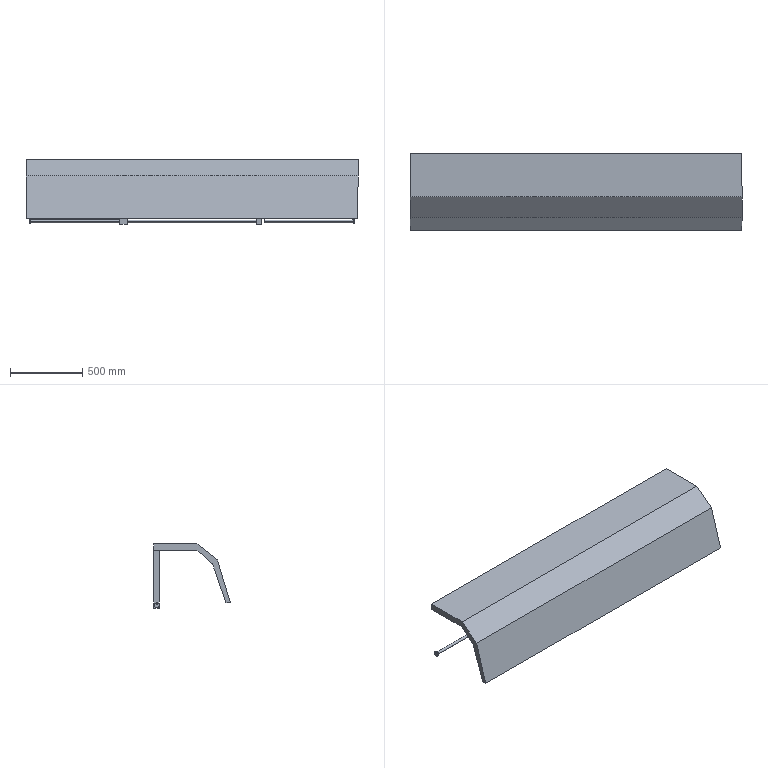Part | SolidWorks | features Cut 2, ICE 2, MirrorPattern 1, MoveFace 1, SplitBody 1 | 2 solids | 39 faces | box 2300 x 530.953 x 444.384 mm | volume 70923348 mm3 | plane 25 | cylinder 14 | commonest cylinder face diameters 20 x6 10 x4 34 x4
STEP:
#1=CARTESIAN_POINT('',(-1113.26,-167.7,-171.172));
#2=VERTEX_POINT('',#1);
#3=CARTESIAN_POINT('',(-1113.26,-163.612,-173.294));
#4=VERTEX_POINT('',#3);
#5=CARTESIAN_POINT('',(-1113.26,-163.612,-168.294));
#6=DIRECTION('',(1.,0.,0.));
#7=DIRECTION('',(0.,0.,-1.));
#8=AXIS2_PLACEMENT_3D('',#5,#6,#7);
#9=CIRCLE('',#8,5.);
#10=EDGE_CURVE('',#2,#4,#9,.T.);
#11=ORIENTED_EDGE('',*,*,#10,.T.);
#12=CARTESIAN_POINT('',(-1127.26,-163.612,-173.294));
#13=VERTEX_POINT('',#12);
#14=CARTESIAN_POINT('',(-1113.26,-163.612,-173.294));
#15=DIRECTION('',(-1.,0.,0.));
#16=VECTOR('',#15,1000.);
#17=LINE('',#14,#16);
#18=EDGE_CURVE('',#4,#13,#17,.T.);
#19=ORIENTED_EDGE('',*,*,#18,.T.);
#20=CARTESIAN_POINT('',(-1127.26,-163.612,-163.294));
#21=VERTEX_POINT('',#20);
#22=CARTESIAN_POINT('',(-1127.26,-163.612,-168.294));
#23=DIRECTION('',(1.,0.,0.));
#24=DIRECTION('',(0.,0.,-1.));
#25=AXIS2_PLACEMENT_3D('',#22,#23,#24);
#26=CIRCLE('',#25,5.);
#27=EDGE_CURVE('',#21,#13,#26,.T.);
#28=ORIENTED_EDGE('',*,*,#27,.F.);
#29=CARTESIAN_POINT('',(-1117.26,-163.612,-163.294));
#30=VERTEX_POINT('',#29);
#31=CARTESIAN_POINT('',(-1113.26,-163.612,-163.294));
#32=DIRECTION('',(-1.,0.,0.));
#33=VECTOR('',#32,1000.);
#34=LINE('',#31,#33);
#35=EDGE_CURVE('',#30,#21,#34,.T.);
#36=ORIENTED_EDGE('',*,*,#35,.F.);
#37=CARTESIAN_POINT('',(-1117.26,-167.7,-171.172));
#38=VERTEX_POINT('',#37);
#39=CARTESIAN_POINT('',(-1117.26,-163.612,-168.294));
#40=DIRECTION('',(1.,0.,0.));
#41=DIRECTION('',(0.,0.,1.));
#42=AXIS2_PLACEMENT_3D('',#39,#40,#41);
#43=CIRCLE('',#42,5.);
#44=EDGE_CURVE('',#30,#38,#43,.T.);
#45=ORIENTED_EDGE('',*,*,#44,.T.);
#46=CARTESIAN_POINT('',(-1120.26,-167.7,-171.172));
#47=DIRECTION('',(-1.,0.,0.));
#48=VECTOR('',#47,1000.);
#49=LINE('',#46,#48);
#50=EDGE_CURVE('',#2,#38,#49,.T.);
#51=ORIENTED_EDGE('',*,*,#50,.F.);
#52=EDGE_LOOP('',(#11,#19,#28,#36,#45,#51));
#53=FACE_OUTER_BOUND('',#52,.T.);
#54=CARTESIAN_POINT('',(-1113.26,-163.612,-168.294));
#55=DIRECTION('',(-1.,0.,0.));
#56=DIRECTION('',(0.,0.,1.));
#57=AXIS2_PLACEMENT_3D('',#54,#55,#56);
#58=CYLINDRICAL_SURFACE('',#57,5.);
#59=ADVANCED_FACE('',(#53),#58,.F.);
#60=CARTESIAN_POINT('',(-1127.26,-163.3,-197.152));
#61=VERTEX_POINT('',#60);
#62=CARTESIAN_POINT('',(-1127.26,-163.3,-163.152));
#63=VERTEX_POINT('',#62);
#64=CARTESIAN_POINT('',(-1127.26,-163.3,-180.152));
#65=DIRECTION('',(1.,0.,0.));
#66=DIRECTION('',(0.,0.,-1.));
#67=AXIS2_PLACEMENT_3D('',#64,#65,#66);
#68=CIRCLE('',#67,17.);
#69=EDGE_CURVE('',#61,#63,#68,.T.);
#70=ORIENTED_EDGE('',*,*,#69,.T.);
#71=CARTESIAN_POINT('',(-1117.26,-163.3,-163.152));
#72=VERTEX_POINT('',#71);
#73=CARTESIAN_POINT('',(-1127.26,-163.3,-163.152));
#74=DIRECTION('',(1.,0.,0.));
#75=VECTOR('',#74,1000.);
#76=LINE('',#73,#75);
#77=EDGE_CURVE('',#63,#72,#76,.T.);
#78=ORIENTED_EDGE('',*,*,#77,.T.);
#79=CARTESIAN_POINT('',(-1117.26,-163.3,-197.152));
#80=VERTEX_POINT('',#79);
#81=CARTESIAN_POINT('',(-1117.26,-163.3,-180.152));
#82=DIRECTION('',(1.,0.,0.));
#83=DIRECTION('',(0.,0.,-1.));
#84=AXIS2_PLACEMENT_3D('',#81,#82,#83);
#85=CIRCLE('',#84,17.);
#86=EDGE_CURVE('',#80,#72,#85,.T.);
#87=ORIENTED_EDGE('',*,*,#86,.F.);
#88=CARTESIAN_POINT('',(-1127.26,-163.3,-197.152));
#89=DIRECTION('',(1.,0.,0.));
#90=VECTOR('',#89,1000.);
#91=LINE('',#88,#90);
#92=EDGE_CURVE('',#61,#80,#91,.T.);
#93=ORIENTED_EDGE('',*,*,#92,.F.);
#94=EDGE_LOOP('',(#70,#78,#87,#93));
#95=FACE_OUTER_BOUND('',#94,.T.);
#96=CARTESIAN_POINT('',(-1127.26,-163.3,-180.152));
#97=DIRECTION('',(1.,0.,0.));
#98=DIRECTION('',(0.,0.,-1.));
#99=AXIS2_PLACEMENT_3D('',#96,#97,#98);
#100=CYLINDRICAL_SURFACE('',#99,17.);
#101=ADVANCED_FACE('',(#95),#100,.T.);
#102=CARTESIAN_POINT('',(-449.45,-153.3,-180.152));
#103=VERTEX_POINT('',#102);
#104=CARTESIAN_POINT('',(-449.45,-173.3,-180.152));
#105=VERTEX_POINT('',#104);
#106=CARTESIAN_POINT('',(-449.45,-163.3,-180.152));
#107=DIRECTION('',(1.,0.,0.));
#108=DIRECTION('',(0.,1.,0.));
#109=AXIS2_PLACEMENT_3D('',#106,#107,#108);
#110=CIRCLE('',#109,10.);
#111=EDGE_CURVE('',#103,#105,#110,.T.);
#112=ORIENTED_EDGE('',*,*,#111,.T.);
#113=CARTESIAN_POINT('',(449.45,-173.3,-180.152));
#114=VERTEX_POINT('',#113);
#115=CARTESIAN_POINT('',(-1178.284,-173.3,-180.152));
#116=DIRECTION('',(1.,0.,0.));
#117=VECTOR('',#116,1000.);
#118=LINE('',#115,#117);
#119=EDGE_CURVE('',#105,#114,#118,.T.);
#120=ORIENTED_EDGE('',*,*,#119,.T.);
#121=CARTESIAN_POINT('',(449.45,-153.3,-180.152));
#122=VERTEX_POINT('',#121);
#123=CARTESIAN_POINT('',(449.45,-163.3,-180.152));
#124=DIRECTION('',(1.,0.,0.));
#125=DIRECTION('',(0.,1.,0.));
#126=AXIS2_PLACEMENT_3D('',#123,#124,#125);
#127=CIRCLE('',#126,10.);
#128=EDGE_CURVE('',#122,#114,#127,.T.);
#129=ORIENTED_EDGE('',*,*,#128,.F.);
#130=CARTESIAN_POINT('',(-1178.284,-153.3,-180.152));
#131=DIRECTION('',(1.,0.,0.));
#132=VECTOR('',#131,1000.);
#133=LINE('',#130,#132);
#134=EDGE_CURVE('',#103,#122,#133,.T.);
#135=ORIENTED_EDGE('',*,*,#134,.F.);
#136=EDGE_LOOP('',(#112,#120,#129,#135));
#137=FACE_OUTER_BOUND('',#136,.T.);
#138=CARTESIAN_POINT('',(-1178.284,-163.3,-180.152));
#139=DIRECTION('',(1.,0.,0.));
#140=DIRECTION('',(0.,1.,0.));
#141=AXIS2_PLACEMENT_3D('',#138,#139,#140);
#142=CYLINDRICAL_SURFACE('',#141,10.);
#143=ADVANCED_FACE('',(#137),#142,.T.);
#144=CARTESIAN_POINT('',(-1117.26,-173.3,-180.152));
#145=VERTEX_POINT('',#144);
#146=CARTESIAN_POINT('',(-1117.26,-163.3,-180.152));
#147=DIRECTION('',(1.,0.,0.));
#148=DIRECTION('',(0.,0.,1.));
#149=AXIS2_PLACEMENT_3D('',#146,#147,#148);
#150=CIRCLE('',#149,10.);
#151=EDGE_CURVE('',#38,#145,#150,.T.);
#152=ORIENTED_EDGE('',*,*,#151,.T.);
#153=CARTESIAN_POINT('',(-499.45,-173.3,-180.152));
#154=VERTEX_POINT('',#153);
#155=CARTESIAN_POINT('',(-1178.284,-173.3,-180.152));
#156=DIRECTION('',(1.,0.,0.));
#157=VECTOR('',#156,1000.);
#158=LINE('',#155,#157);
#159=EDGE_CURVE('',#145,#154,#158,.T.);
#160=ORIENTED_EDGE('',*,*,#159,.T.);
#161=CARTESIAN_POINT('',(-499.45,-153.3,-180.152));
#162=VERTEX_POINT('',#161);
#163=CARTESIAN_POINT('',(-499.45,-163.3,-180.152));
#164=DIRECTION('',(-1.,0.,0.));
#165=DIRECTION('',(0.,1.,0.));
#166=AXIS2_PLACEMENT_3D('',#163,#164,#165);
#167=CIRCLE('',#166,10.);
#168=EDGE_CURVE('',#154,#162,#167,.T.);
#169=ORIENTED_EDGE('',*,*,#168,.T.);
#170=CARTESIAN_POINT('',(-1117.26,-153.3,-180.152));
#171=VERTEX_POINT('',#170);
#172=CARTESIAN_POINT('',(-1178.284,-153.3,-180.152));
#173=DIRECTION('',(1.,0.,0.));
#174=VECTOR('',#173,1000.);
#175=LINE('',#172,#174);
#176=EDGE_CURVE('',#171,#162,#175,.T.);
#177=ORIENTED_EDGE('',*,*,#176,.F.);
#178=CARTESIAN_POINT('',(-1117.26,-159.378,-170.953));
#179=VERTEX_POINT('',#178);
#180=CARTESIAN_POINT('',(-1117.26,-163.3,-180.152));
#181=DIRECTION('',(1.,0.,0.));
#182=DIRECTION('',(0.,0.,1.));
#183=AXIS2_PLACEMENT_3D('',#180,#181,#182);
#184=CIRCLE('',#183,10.);
#185=EDGE_CURVE('',#171,#179,#184,.T.);
#186=ORIENTED_EDGE('',*,*,#185,.T.);
#187=CARTESIAN_POINT('',(-1113.26,-159.378,-170.953));
#188=VERTEX_POINT('',#187);
#189=CARTESIAN_POINT('',(-1120.26,-159.378,-170.953));
#190=DIRECTION('',(1.,0.,0.));
#191=VECTOR('',#190,1000.);
#192=LINE('',#189,#191);
#193=EDGE_CURVE('',#179,#188,#192,.T.);
#194=ORIENTED_EDGE('',*,*,#193,.T.);
#195=CARTESIAN_POINT('',(-1113.26,-163.3,-180.152));
#196=DIRECTION('',(1.,0.,0.));
#197=DIRECTION('',(0.,0.,1.));
#198=AXIS2_PLACEMENT_3D('',#195,#196,#197);
#199=CIRCLE('',#198,10.);
#200=EDGE_CURVE('',#188,#2,#199,.T.);
#201=ORIENTED_EDGE('',*,*,#200,.T.);
#202=ORIENTED_EDGE('',*,*,#50,.T.);
#203=EDGE_LOOP('',(#152,#160,#169,#177,#186,#194,#201,#202));
#204=FACE_OUTER_BOUND('',#203,.T.);
#205=CARTESIAN_POINT('',(-1178.284,-163.3,-180.152));
#206=DIRECTION('',(1.,0.,0.));
#207=DIRECTION('',(0.,1.,0.));
#208=AXIS2_PLACEMENT_3D('',#205,#206,#207);
#209=CYLINDRICAL_SURFACE('',#208,10.);
#210=ADVANCED_FACE('',(#204),#209,.T.);
#211=CARTESIAN_POINT('',(449.45,-141.634,-200.));
#212=VERTEX_POINT('',#211);
#213=CARTESIAN_POINT('',(484.45,-141.634,-200.));
#214=VERTEX_POINT('',#213);
#215=CARTESIAN_POINT('',(0.,-141.634,-200.));
#216=DIRECTION('',(1.,0.,0.));
#217=VECTOR('',#216,1000.);
#218=LINE('',#215,#217);
#219=EDGE_CURVE('',#212,#214,#218,.T.);
#220=ORIENTED_EDGE('',*,*,#219,.T.);
#221=CARTESIAN_POINT('',(484.45,-181.634,-200.));
#222=VERTEX_POINT('',#221);
#223=CARTESIAN_POINT('',(484.45,-181.634,-200.));
#224=DIRECTION('',(0.,1.,0.));
#225=VECTOR('',#224,1000.);
#226=LINE('',#223,#225);
#227=EDGE_CURVE('',#222,#214,#226,.T.);
#228=ORIENTED_EDGE('',*,*,#227,.F.);
#229=CARTESIAN_POINT('',(449.45,-181.634,-200.));
#230=VERTEX_POINT('',#229);
#231=CARTESIAN_POINT('',(499.45,-181.634,-200.));
#232=DIRECTION('',(-1.,0.,0.));
#233=VECTOR('',#232,1000.);
#234=LINE('',#231,#233);
#235=EDGE_CURVE('',#222,#230,#234,.T.);
#236=ORIENTED_EDGE('',*,*,#235,.T.);
#237=CARTESIAN_POINT('',(449.45,0.,-200.));
#238=DIRECTION('',(0.,-1.,0.));
#239=VECTOR('',#238,1000.);
#240=LINE('',#237,#239);
#241=EDGE_CURVE('',#212,#230,#240,.T.);
#242=ORIENTED_EDGE('',*,*,#241,.F.);
#243=EDGE_LOOP('',(#220,#228,#236,#242));
#244=FACE_OUTER_BOUND('',#243,.T.);
#245=CARTESIAN_POINT('',(0.,0.,-200.));
#246=DIRECTION('',(0.,0.,-1.));
#247=DIRECTION('',(-1.,0.,0.));
#248=AXIS2_PLACEMENT_3D('',#245,#246,#247);
#249=PLANE('',#248);
#250=ADVANCED_FACE('',(#244),#249,.T.);
#251=CARTESIAN_POINT('',(484.45,-181.634,200.));
#252=VERTEX_POINT('',#251);
#253=CARTESIAN_POINT('',(484.45,-181.634,200.));
#254=DIRECTION('',(0.,0.,-1.));
#255=VECTOR('',#254,1000.);
#256=LINE('',#253,#255);
#257=EDGE_CURVE('',#252,#222,#256,.T.);
#258=ORIENTED_EDGE('',*,*,#257,.F.);
#259=CARTESIAN_POINT('',(449.45,-181.634,200.));
#260=VERTEX_POINT('',#259);
#261=CARTESIAN_POINT('',(-1150.,-181.634,200.));
#262=DIRECTION('',(-1.,0.,0.));
#263=VECTOR('',#262,1000.);
#264=LINE('',#261,#263);
#265=EDGE_CURVE('',#252,#260,#264,.T.);
#266=ORIENTED_EDGE('',*,*,#265,.T.);
#267=CARTESIAN_POINT('',(449.45,-181.634,40.));
#268=DIRECTION('',(0.,0.,1.));
#269=VECTOR('',#268,1000.);
#270=LINE('',#267,#269);
#271=EDGE_CURVE('',#230,#260,#270,.T.);
#272=ORIENTED_EDGE('',*,*,#271,.F.);
#273=ORIENTED_EDGE('',*,*,#235,.F.);
#274=EDGE_LOOP('',(#258,#266,#272,#273));
#275=FACE_OUTER_BOUND('',#274,.T.);
#276=CARTESIAN_POINT('',(499.45,-181.634,-200.));
#277=DIRECTION('',(0.,1.,0.));
#278=DIRECTION('',(0.,0.,1.));
#279=AXIS2_PLACEMENT_3D('',#276,#277,#278);
#280=PLANE('',#279);
#281=ADVANCED_FACE('',(#275),#280,.F.);
#282=ORIENTED_EDGE('',*,*,#159,.F.);
#283=CARTESIAN_POINT('',(-1117.26,-163.3,-180.152));
#284=DIRECTION('',(1.,0.,0.));
#285=DIRECTION('',(0.,0.,1.));
#286=AXIS2_PLACEMENT_3D('',#283,#284,#285);
#287=CIRCLE('',#286,10.);
#288=EDGE_CURVE('',#145,#171,#287,.T.);
#289=ORIENTED_EDGE('',*,*,#288,.T.);
#290=ORIENTED_EDGE('',*,*,#176,.T.);
#291=CARTESIAN_POINT('',(-499.45,-163.3,-180.152));
#292=DIRECTION('',(-1.,0.,0.));
#293=DIRECTION('',(0.,1.,0.));
#294=AXIS2_PLACEMENT_3D('',#291,#292,#293);
#295=CIRCLE('',#294,10.);
#296=EDGE_CURVE('',#162,#154,#295,.T.);
#297=ORIENTED_EDGE('',*,*,#296,.T.);
#298=EDGE_LOOP('',(#282,#289,#290,#297));
#299=FACE_OUTER_BOUND('',#298,.T.);
#300=CARTESIAN_POINT('',(-1178.284,-163.3,-180.152));
#301=DIRECTION('',(1.,0.,0.));
#302=DIRECTION('',(0.,1.,0.));
#303=AXIS2_PLACEMENT_3D('',#300,#301,#302);
#304=CYLINDRICAL_SURFACE('',#303,10.);
#305=ADVANCED_FACE('',(#299),#304,.T.);
#306=CARTESIAN_POINT('',(1150.,-641.958,-163.652));
#307=VERTEX_POINT('',#306);
#308=CARTESIAN_POINT('',(1150.,-549.64,105.835));
#309=VERTEX_POINT('',#308);
#310=CARTESIAN_POINT('',(1150.,-641.958,-163.652));
#311=DIRECTION('',(0.,0.3241,0.946));
#312=VECTOR('',#311,1000.);
#313=LINE('',#310,#312);
#314=EDGE_CURVE('',#307,#309,#313,.T.);
#315=ORIENTED_EDGE('',*,*,#314,.T.);
#316=CARTESIAN_POINT('',(1150.,-441.634,200.));
#317=VERTEX_POINT('',#316);
#318=CARTESIAN_POINT('',(1150.,-549.64,105.835));
#319=DIRECTION('',(0.,0.7538,0.6572));
#320=VECTOR('',#319,1000.);
#321=LINE('',#318,#320);
#322=EDGE_CURVE('',#309,#317,#321,.T.);
#323=ORIENTED_EDGE('',*,*,#322,.T.);
#324=CARTESIAN_POINT('',(1150.,-141.634,200.));
#325=VERTEX_POINT('',#324);
#326=CARTESIAN_POINT('',(1150.,0.,200.));
#327=DIRECTION('',(0.,1.,0.));
#328=VECTOR('',#327,1000.);
#329=LINE('',#326,#328);
#330=EDGE_CURVE('',#317,#325,#329,.T.);
#331=ORIENTED_EDGE('',*,*,#330,.T.);
#332=CARTESIAN_POINT('',(1150.,-141.634,244.384));
#333=VERTEX_POINT('',#332);
#334=CARTESIAN_POINT('',(1150.,-141.634,0.));
#335=DIRECTION('',(0.,0.,1.));
#336=VECTOR('',#335,1000.);
#337=LINE('',#334,#336);
#338=EDGE_CURVE('',#325,#333,#337,.T.);
#339=ORIENTED_EDGE('',*,*,#338,.T.);
#340=CARTESIAN_POINT('',(1150.,-441.634,244.384));
#341=VERTEX_POINT('',#340);
#342=CARTESIAN_POINT('',(1150.,0.,244.384));
#343=DIRECTION('',(0.,-1.,0.));
#344=VECTOR('',#343,1000.);
#345=LINE('',#342,#344);
#346=EDGE_CURVE('',#333,#341,#345,.T.);
#347=ORIENTED_EDGE('',*,*,#346,.T.);
#348=CARTESIAN_POINT('',(1150.,-583.719,133.154));
#349=VERTEX_POINT('',#348);
#350=CARTESIAN_POINT('',(1150.,-286.429,365.884));
#351=DIRECTION('',(0.,0.7874,0.6164));
#352=VECTOR('',#351,1000.);
#353=LINE('',#350,#352);
#354=EDGE_CURVE('',#349,#341,#353,.T.);
#355=ORIENTED_EDGE('',*,*,#354,.F.);
#356=CARTESIAN_POINT('',(1150.,-672.587,-163.652));
#357=VERTEX_POINT('',#356);
#358=CARTESIAN_POINT('',(1150.,-572.282,171.349));
#359=DIRECTION('',(0.,0.2868,0.958));
#360=VECTOR('',#359,1000.);
#361=LINE('',#358,#360);
#362=EDGE_CURVE('',#357,#349,#361,.T.);
#363=ORIENTED_EDGE('',*,*,#362,.F.);
#364=CARTESIAN_POINT('',(1150.,0.,-163.652));
#365=DIRECTION('',(0.,1.,0.));
#366=VECTOR('',#365,1000.);
#367=LINE('',#364,#366);
#368=EDGE_CURVE('',#357,#307,#367,.T.);
#369=ORIENTED_EDGE('',*,*,#368,.T.);
#370=EDGE_LOOP('',(#315,#323,#331,#339,#347,#355,#363,#369));
#371=FACE_OUTER_BOUND('',#370,.T.);
#372=CARTESIAN_POINT('',(1150.,0.,0.));
#373=DIRECTION('',(1.,0.,0.));
#374=DIRECTION('',(0.,0.,-1.));
#375=AXIS2_PLACEMENT_3D('',#372,#373,#374);
#376=PLANE('',#375);
#377=ADVANCED_FACE('',(#371),#376,.T.);
#378=CARTESIAN_POINT('',(-1150.,-549.64,105.835));
#379=VERTEX_POINT('',#378);
#380=CARTESIAN_POINT('',(-1150.,-441.634,200.));
#381=VERTEX_POINT('',#380);
#382=CARTESIAN_POINT('',(-1150.,-549.64,105.835));
#383=DIRECTION('',(0.,0.7538,0.6572));
#384=VECTOR('',#383,1000.);
#385=LINE('',#382,#384);
#386=EDGE_CURVE('',#379,#381,#385,.T.);
#387=ORIENTED_EDGE('',*,*,#386,.F.);
#388=CARTESIAN_POINT('',(-1150.,-641.958,-163.652));
#389=VERTEX_POINT('',#388);
#390=CARTESIAN_POINT('',(-1150.,-641.958,-163.652));
#391=DIRECTION('',(0.,0.3241,0.946));
#392=VECTOR('',#391,1000.);
#393=LINE('',#390,#392);
#394=EDGE_CURVE('',#389,#379,#393,.T.);
#395=ORIENTED_EDGE('',*,*,#394,.F.);
#396=CARTESIAN_POINT('',(-1150.,-672.587,-163.652));
#397=VERTEX_POINT('',#396);
#398=CARTESIAN_POINT('',(-1150.,0.,-163.652));
#399=DIRECTION('',(0.,-1.,0.));
#400=VECTOR('',#399,1000.);
#401=LINE('',#398,#400);
#402=EDGE_CURVE('',#389,#397,#401,.T.);
#403=ORIENTED_EDGE('',*,*,#402,.T.);
#404=CARTESIAN_POINT('',(-1150.,-583.719,133.154));
#405=VERTEX_POINT('',#404);
#406=CARTESIAN_POINT('',(-1150.,-572.282,171.349));
#407=DIRECTION('',(0.,-0.2868,-0.958));
#408=VECTOR('',#407,1000.);
#409=LINE('',#406,#408);
#410=EDGE_CURVE('',#405,#397,#409,.T.);
#411=ORIENTED_EDGE('',*,*,#410,.F.);
#412=CARTESIAN_POINT('',(-1150.,-441.634,244.384));
#413=VERTEX_POINT('',#412);
#414=CARTESIAN_POINT('',(-1150.,-441.634,244.384));
#415=DIRECTION('',(0.,-0.7874,-0.6164));
#416=VECTOR('',#415,1000.);
#417=LINE('',#414,#416);
#418=EDGE_CURVE('',#413,#405,#417,.T.);
#419=ORIENTED_EDGE('',*,*,#418,.F.);
#420=CARTESIAN_POINT('',(-1150.,-141.634,244.384));
#421=VERTEX_POINT('',#420);
#422=CARTESIAN_POINT('',(-1150.,0.,244.384));
#423=DIRECTION('',(0.,-1.,0.));
#424=VECTOR('',#423,1000.);
#425=LINE('',#422,#424);
#426=EDGE_CURVE('',#421,#413,#425,.T.);
#427=ORIENTED_EDGE('',*,*,#426,.F.);
#428=CARTESIAN_POINT('',(-1150.,-141.634,200.));
#429=VERTEX_POINT('',#428);
#430=CARTESIAN_POINT('',(-1150.,-141.634,0.));
#431=DIRECTION('',(0.,0.,1.));
#432=VECTOR('',#431,1000.);
#433=LINE('',#430,#432);
#434=EDGE_CURVE('',#429,#421,#433,.T.);
#435=ORIENTED_EDGE('',*,*,#434,.F.);
#436=CARTESIAN_POINT('',(-1150.,0.,200.));
#437=DIRECTION('',(0.,1.,0.));
#438=VECTOR('',#437,1000.);
#439=LINE('',#436,#438);
#440=EDGE_CURVE('',#381,#429,#439,.T.);
#441=ORIENTED_EDGE('',*,*,#440,.F.);
#442=EDGE_LOOP('',(#387,#395,#403,#411,#419,#427,#435,#441));
#443=FACE_OUTER_BOUND('',#442,.T.);
#444=CARTESIAN_POINT('',(-1150.,0.,0.));
#445=DIRECTION('',(1.,0.,0.));
#446=DIRECTION('',(0.,0.,-1.));
#447=AXIS2_PLACEMENT_3D('',#444,#445,#446);
#448=PLANE('',#447);
#449=ADVANCED_FACE('',(#443),#448,.F.);
#450=CARTESIAN_POINT('',(-1150.,-549.64,105.835));
#451=DIRECTION('',(-1.,0.,0.));
#452=VECTOR('',#451,1000.);
#453=LINE('',#450,#452);
#454=EDGE_CURVE('',#309,#379,#453,.T.);
#455=ORIENTED_EDGE('',*,*,#454,.T.);
#456=ORIENTED_EDGE('',*,*,#386,.T.);
#457=CARTESIAN_POINT('',(-1150.,-441.634,200.));
#458=DIRECTION('',(1.,0.,0.));
#459=VECTOR('',#458,1000.);
#460=LINE('',#457,#459);
#461=EDGE_CURVE('',#381,#317,#460,.T.);
#462=ORIENTED_EDGE('',*,*,#461,.T.);
#463=ORIENTED_EDGE('',*,*,#322,.F.);
#464=EDGE_LOOP('',(#455,#456,#462,#463));
#465=FACE_OUTER_BOUND('',#464,.T.);
#466=CARTESIAN_POINT('',(-1150.,-289.789,332.385));
#467=DIRECTION('',(0.,-0.6572,0.7538));
#468=DIRECTION('',(0.,-0.7538,-0.6572));
#469=AXIS2_PLACEMENT_3D('',#466,#467,#468);
#470=PLANE('',#469);
#471=ADVANCED_FACE('',(#465),#470,.F.);
#472=CARTESIAN_POINT('',(-1150.,-641.958,-163.652));
#473=DIRECTION('',(-1.,0.,0.));
#474=VECTOR('',#473,1000.);
#475=LINE('',#472,#474);
#476=EDGE_CURVE('',#307,#389,#475,.T.);
#477=ORIENTED_EDGE('',*,*,#476,.T.);
#478=ORIENTED_EDGE('',*,*,#394,.T.);
#479=ORIENTED_EDGE('',*,*,#454,.F.);
#480=ORIENTED_EDGE('',*,*,#314,.F.);
#481=EDGE_LOOP('',(#477,#478,#479,#480));
#482=FACE_OUTER_BOUND('',#481,.T.);
#483=CARTESIAN_POINT('',(-1150.,-524.361,179.629));
#484=DIRECTION('',(0.,-0.946,0.3241));
#485=DIRECTION('',(0.,-0.3241,-0.946));
#486=AXIS2_PLACEMENT_3D('',#483,#484,#485);
#487=PLANE('',#486);
#488=ADVANCED_FACE('',(#482),#487,.F.);
#489=CARTESIAN_POINT('',(-1150.,-672.587,-163.652));
#490=DIRECTION('',(1.,0.,0.));
#491=VECTOR('',#490,1000.);
#492=LINE('',#489,#491);
#493=EDGE_CURVE('',#397,#357,#492,.T.);
#494=ORIENTED_EDGE('',*,*,#493,.F.);
#495=ORIENTED_EDGE('',*,*,#402,.F.);
#496=ORIENTED_EDGE('',*,*,#476,.F.);
#497=ORIENTED_EDGE('',*,*,#368,.F.);
#498=EDGE_LOOP('',(#494,#495,#496,#497));
#499=FACE_OUTER_BOUND('',#498,.T.);
#500=CARTESIAN_POINT('',(-1150.,0.,-163.652));
#501=DIRECTION('',(0.,0.,1.));
#502=DIRECTION('',(1.,0.,0.));
#503=AXIS2_PLACEMENT_3D('',#500,#501,#502);
#504=PLANE('',#503);
#505=ADVANCED_FACE('',(#499),#504,.F.);
#506=ORIENTED_EDGE('',*,*,#410,.T.);
#507=ORIENTED_EDGE('',*,*,#493,.T.);
#508=ORIENTED_EDGE('',*,*,#362,.T.);
#509=CARTESIAN_POINT('',(-1150.,-583.719,133.154));
#510=DIRECTION('',(-1.,0.,0.));
#511=VECTOR('',#510,1000.);
#512=LINE('',#509,#511);
#513=EDGE_CURVE('',#349,#405,#512,.T.);
#514=ORIENTED_EDGE('',*,*,#513,.T.);
#515=EDGE_LOOP('',(#506,#507,#508,#514));
#516=FACE_OUTER_BOUND('',#515,.T.);
#517=CARTESIAN_POINT('',(-1150.,-572.282,171.349));
#518=DIRECTION('',(0.,-0.958,0.2868));
#519=DIRECTION('',(0.,-0.2868,-0.958));
#520=AXIS2_PLACEMENT_3D('',#517,#518,#519);
#521=PLANE('',#520);
#522=ADVANCED_FACE('',(#516),#521,.T.);
#523=ORIENTED_EDGE('',*,*,#418,.T.);
#524=ORIENTED_EDGE('',*,*,#513,.F.);
#525=ORIENTED_EDGE('',*,*,#354,.T.);
#526=CARTESIAN_POINT('',(-1150.,-441.634,244.384));
#527=DIRECTION('',(-1.,0.,0.));
#528=VECTOR('',#527,1000.);
#529=LINE('',#526,#528);
#530=EDGE_CURVE('',#341,#413,#529,.T.);
#531=ORIENTED_EDGE('',*,*,#530,.T.);
#532=EDGE_LOOP('',(#523,#524,#525,#531));
#533=FACE_OUTER_BOUND('',#532,.T.);
#534=CARTESIAN_POINT('',(-1150.,-286.429,365.884));
#535=DIRECTION('',(0.,-0.6164,0.7874));
#536=DIRECTION('',(0.,-0.7874,-0.6164));
#537=AXIS2_PLACEMENT_3D('',#534,#535,#536);
#538=PLANE('',#537);
#539=ADVANCED_FACE('',(#533),#538,.T.);
#540=ORIENTED_EDGE('',*,*,#426,.T.);
#541=ORIENTED_EDGE('',*,*,#530,.F.);
#542=ORIENTED_EDGE('',*,*,#346,.F.);
#543=CARTESIAN_POINT('',(-1150.,-141.634,244.384));
#544=DIRECTION('',(-1.,0.,0.));
#545=VECTOR('',#544,1000.);
#546=LINE('',#543,#545);
#547=EDGE_CURVE('',#333,#421,#546,.T.);
#548=ORIENTED_EDGE('',*,*,#547,.T.);
#549=EDGE_LOOP('',(#540,#541,#542,#548));
#550=FACE_OUTER_BOUND('',#549,.T.);
#551=CARTESIAN_POINT('',(-1150.,0.,244.384));
#552=DIRECTION('',(0.,0.,1.));
#553=DIRECTION('',(1.,0.,0.));
#554=AXIS2_PLACEMENT_3D('',#551,#552,#553);
#555=PLANE('',#554);
#556=ADVANCED_FACE('',(#550),#555,.T.);
#557=ORIENTED_EDGE('',*,*,#265,.F.);
#558=CARTESIAN_POINT('',(484.45,-141.634,200.));
#559=VERTEX_POINT('',#558);
#560=CARTESIAN_POINT('',(484.45,-141.634,200.));
#561=DIRECTION('',(0.,-1.,0.));
#562=VECTOR('',#561,1000.);
#563=LINE('',#560,#562);
#564=EDGE_CURVE('',#559,#252,#563,.T.);
#565=ORIENTED_EDGE('',*,*,#564,.F.);
#566=CARTESIAN_POINT('',(-1150.,-141.634,200.));
#567=DIRECTION('',(-1.,0.,0.));
#568=VECTOR('',#567,1000.);
#569=LINE('',#566,#568);
#570=EDGE_CURVE('',#325,#559,#569,.T.);
#571=ORIENTED_EDGE('',*,*,#570,.F.);
#572=ORIENTED_EDGE('',*,*,#330,.F.);
#573=ORIENTED_EDGE('',*,*,#461,.F.);
#574=ORIENTED_EDGE('',*,*,#440,.T.);
#575=CARTESIAN_POINT('',(-499.45,-141.634,200.));
#576=VERTEX_POINT('',#575);
#577=CARTESIAN_POINT('',(-1150.,-141.634,200.));
#578=DIRECTION('',(-1.,0.,0.));
#579=VECTOR('',#578,1000.);
#580=LINE('',#577,#579);
#581=EDGE_CURVE('',#576,#429,#580,.T.);
#582=ORIENTED_EDGE('',*,*,#581,.F.);
#583=CARTESIAN_POINT('',(-499.45,-181.634,200.));
#584=VERTEX_POINT('',#583);
#585=CARTESIAN_POINT('',(-499.45,0.,200.));
#586=DIRECTION('',(0.,1.,0.));
#587=VECTOR('',#586,1000.);
#588=LINE('',#585,#587);
#589=EDGE_CURVE('',#584,#576,#588,.T.);
#590=ORIENTED_EDGE('',*,*,#589,.F.);
#591=CARTESIAN_POINT('',(-449.45,-181.634,200.));
#592=VERTEX_POINT('',#591);
#593=CARTESIAN_POINT('',(-1150.,-181.634,200.));
#594=DIRECTION('',(-1.,0.,0.));
#595=VECTOR('',#594,1000.);
#596=LINE('',#593,#595);
#597=EDGE_CURVE('',#592,#584,#596,.T.);
#598=ORIENTED_EDGE('',*,*,#597,.F.);
#599=CARTESIAN_POINT('',(-449.45,-141.634,200.));
#600=VERTEX_POINT('',#599);
#601=CARTESIAN_POINT('',(-449.45,0.,200.));
#602=DIRECTION('',(0.,-1.,0.));
#603=VECTOR('',#602,1000.);
#604=LINE('',#601,#603);
#605=EDGE_CURVE('',#600,#592,#604,.T.);
#606=ORIENTED_EDGE('',*,*,#605,.F.);
#607=CARTESIAN_POINT('',(449.45,-141.634,200.));
#608=VERTEX_POINT('',#607);
#609=CARTESIAN_POINT('',(-1150.,-141.634,200.));
#610=DIRECTION('',(-1.,0.,0.));
#611=VECTOR('',#610,1000.);
#612=LINE('',#609,#611);
#613=EDGE_CURVE('',#608,#600,#612,.T.);
#614=ORIENTED_EDGE('',*,*,#613,.F.);
#615=CARTESIAN_POINT('',(449.45,0.,200.));
#616=DIRECTION('',(0.,1.,0.));
#617=VECTOR('',#616,1000.);
#618=LINE('',#615,#617);
#619=EDGE_CURVE('',#260,#608,#618,.T.);
#620=ORIENTED_EDGE('',*,*,#619,.F.);
#621=EDGE_LOOP('',(#557,#565,#571,#572,#573,#574,#582,#590,#598,#606,#614,#620));
#622=FACE_OUTER_BOUND('',#621,.T.);
#623=CARTESIAN_POINT('',(-1150.,0.,200.));
#624=DIRECTION('',(0.,0.,1.));
#625=DIRECTION('',(1.,0.,0.));
#626=AXIS2_PLACEMENT_3D('',#623,#624,#625);
#627=PLANE('',#626);
#628=ADVANCED_FACE('',(#622),#627,.F.);
#629=CARTESIAN_POINT('',(-499.45,-141.634,-200.));
#630=VERTEX_POINT('',#629);
#631=CARTESIAN_POINT('',(-499.45,-141.634,-200.));
#632=DIRECTION('',(0.,0.,-1.));
#633=VECTOR('',#632,1000.);
#634=LINE('',#631,#633);
#635=EDGE_CURVE('',#576,#630,#634,.T.);
#636=ORIENTED_EDGE('',*,*,#635,.T.);
#637=CARTESIAN_POINT('',(-499.45,-181.634,-200.));
#638=VERTEX_POINT('',#637);
#639=CARTESIAN_POINT('',(-499.45,0.,-200.));
#640=DIRECTION('',(0.,1.,0.));
#641=VECTOR('',#640,1000.);
#642=LINE('',#639,#641);
#643=EDGE_CURVE('',#638,#630,#642,.T.);
#644=ORIENTED_EDGE('',*,*,#643,.F.);
#645=CARTESIAN_POINT('',(-499.45,-181.634,40.));
#646=DIRECTION('',(0.,0.,-1.));
#647=VECTOR('',#646,1000.);
#648=LINE('',#645,#647);
#649=EDGE_CURVE('',#584,#638,#648,.T.);
#650=ORIENTED_EDGE('',*,*,#649,.F.);
#651=ORIENTED_EDGE('',*,*,#589,.T.);
#652=EDGE_LOOP('',(#636,#644,#650,#651));
#653=FACE_OUTER_BOUND('',#652,.T.);
#654=ORIENTED_EDGE('',*,*,#296,.F.);
#655=ORIENTED_EDGE('',*,*,#168,.F.);
#656=EDGE_LOOP('',(#654,#655));
#657=FACE_BOUND('',#656,.T.);
#658=CARTESIAN_POINT('',(-499.45,0.,40.));
#659=DIRECTION('',(1.,0.,0.));
#660=DIRECTION('',(0.,1.,0.));
#661=AXIS2_PLACEMENT_3D('',#658,#659,#660);
#662=PLANE('',#661);
#663=ADVANCED_FACE('',(#653,#657),#662,.F.);
#664=ORIENTED_EDGE('',*,*,#649,.T.);
#665=CARTESIAN_POINT('',(-449.45,-181.634,-200.));
#666=VERTEX_POINT('',#665);
#667=CARTESIAN_POINT('',(-499.45,-181.634,-200.));
#668=DIRECTION('',(-1.,0.,0.));
#669=VECTOR('',#668,1000.);
#670=LINE('',#667,#669);
#671=EDGE_CURVE('',#666,#638,#670,.T.);
#672=ORIENTED_EDGE('',*,*,#671,.F.);
#673=CARTESIAN_POINT('',(-449.45,-181.634,-200.));
#674=DIRECTION('',(0.,0.,-1.));
#675=VECTOR('',#674,1000.);
#676=LINE('',#673,#675);
#677=EDGE_CURVE('',#592,#666,#676,.T.);
#678=ORIENTED_EDGE('',*,*,#677,.F.);
#679=ORIENTED_EDGE('',*,*,#597,.T.);
#680=EDGE_LOOP('',(#664,#672,#678,#679));
#681=FACE_OUTER_BOUND('',#680,.T.);
#682=CARTESIAN_POINT('',(-499.45,-181.634,-200.));
#683=DIRECTION('',(0.,1.,0.));
#684=DIRECTION('',(0.,0.,1.));
#685=AXIS2_PLACEMENT_3D('',#682,#683,#684);
#686=PLANE('',#685);
#687=ADVANCED_FACE('',(#681),#686,.F.);
#688=CARTESIAN_POINT('',(-449.45,-141.634,-200.));
#689=VERTEX_POINT('',#688);
#690=CARTESIAN_POINT('',(-449.45,0.,-200.));
#691=DIRECTION('',(0.,-1.,0.));
#692=VECTOR('',#691,1000.);
#693=LINE('',#690,#692);
#694=EDGE_CURVE('',#689,#666,#693,.T.);
#695=ORIENTED_EDGE('',*,*,#694,.F.);
#696=CARTESIAN_POINT('',(-449.45,-141.634,-200.));
#697=DIRECTION('',(0.,0.,1.));
#698=VECTOR('',#697,1000.);
#699=LINE('',#696,#698);
#700=EDGE_CURVE('',#689,#600,#699,.T.);
#701=ORIENTED_EDGE('',*,*,#700,.T.);
#702=ORIENTED_EDGE('',*,*,#605,.T.);
#703=ORIENTED_EDGE('',*,*,#677,.T.);
#704=EDGE_LOOP('',(#695,#701,#702,#703));
#705=FACE_OUTER_BOUND('',#704,.T.);
#706=ORIENTED_EDGE('',*,*,#111,.F.);
#707=CARTESIAN_POINT('',(-449.45,-163.3,-180.152));
#708=DIRECTION('',(1.,0.,0.));
#709=DIRECTION('',(0.,1.,0.));
#710=AXIS2_PLACEMENT_3D('',#707,#708,#709);
#711=CIRCLE('',#710,10.);
#712=EDGE_CURVE('',#105,#103,#711,.T.);
#713=ORIENTED_EDGE('',*,*,#712,.F.);
#714=EDGE_LOOP('',(#706,#713));
#715=FACE_BOUND('',#714,.T.);
#716=CARTESIAN_POINT('',(-449.45,0.,40.));
#717=DIRECTION('',(-1.,0.,0.));
#718=DIRECTION('',(0.,0.,1.));
#719=AXIS2_PLACEMENT_3D('',#716,#717,#718);
#720=PLANE('',#719);
#721=ADVANCED_FACE('',(#705,#715),#720,.F.);
#722=CARTESIAN_POINT('',(449.45,-141.634,-200.));
#723=DIRECTION('',(0.,0.,-1.));
#724=VECTOR('',#723,1000.);
#725=LINE('',#722,#724);
#726=EDGE_CURVE('',#608,#212,#725,.T.);
#727=ORIENTED_EDGE('',*,*,#726,.T.);
#728=ORIENTED_EDGE('',*,*,#241,.T.);
#729=ORIENTED_EDGE('',*,*,#271,.T.);
#730=ORIENTED_EDGE('',*,*,#619,.T.);
#731=EDGE_LOOP('',(#727,#728,#729,#730));
#732=FACE_OUTER_BOUND('',#731,.T.);
#733=ORIENTED_EDGE('',*,*,#128,.T.);
#734=CARTESIAN_POINT('',(449.45,-163.3,-180.152));
#735=DIRECTION('',(1.,0.,0.));
#736=DIRECTION('',(0.,1.,0.));
#737=AXIS2_PLACEMENT_3D('',#734,#735,#736);
#738=CIRCLE('',#737,10.);
#739=EDGE_CURVE('',#114,#122,#738,.T.);
#740=ORIENTED_EDGE('',*,*,#739,.T.);
#741=EDGE_LOOP('',(#733,#740));
#742=FACE_BOUND('',#741,.T.);
#743=CARTESIAN_POINT('',(449.45,0.,40.));
#744=DIRECTION('',(-1.,0.,0.));
#745=DIRECTION('',(0.,0.,1.));
#746=AXIS2_PLACEMENT_3D('',#743,#744,#745);
#747=PLANE('',#746);
#748=ADVANCED_FACE('',(#732,#742),#747,.T.);
#749=ORIENTED_EDGE('',*,*,#643,.T.);
#750=CARTESIAN_POINT('',(-499.45,-141.634,-200.));
#751=DIRECTION('',(1.,0.,0.));
#752=VECTOR('',#751,1000.);
#753=LINE('',#750,#752);
#754=EDGE_CURVE('',#630,#689,#753,.T.);
#755=ORIENTED_EDGE('',*,*,#754,.T.);
#756=ORIENTED_EDGE('',*,*,#694,.T.);
#757=ORIENTED_EDGE('',*,*,#671,.T.);
#758=EDGE_LOOP('',(#749,#755,#756,#757));
#759=FACE_OUTER_BOUND('',#758,.T.);
#760=CARTESIAN_POINT('',(0.,0.,-200.));
#761=DIRECTION('',(0.,0.,1.));
#762=DIRECTION('',(1.,0.,0.));
#763=AXIS2_PLACEMENT_3D('',#760,#761,#762);
#764=PLANE('',#763);
#765=ADVANCED_FACE('',(#759),#764,.F.);
#766=ORIENTED_EDGE('',*,*,#119,.F.);
#767=ORIENTED_EDGE('',*,*,#712,.T.);
#768=ORIENTED_EDGE('',*,*,#134,.T.);
#769=ORIENTED_EDGE('',*,*,#739,.F.);
#770=EDGE_LOOP('',(#766,#767,#768,#769));
#771=FACE_OUTER_BOUND('',#770,.T.);
#772=CARTESIAN_POINT('',(-1178.284,-163.3,-180.152));
#773=DIRECTION('',(1.,0.,0.));
#774=DIRECTION('',(0.,1.,0.));
#775=AXIS2_PLACEMENT_3D('',#772,#773,#774);
#776=CYLINDRICAL_SURFACE('',#775,10.);
#777=ADVANCED_FACE('',(#771),#776,.T.);
#778=ORIENTED_EDGE('',*,*,#570,.T.);
#779=CARTESIAN_POINT('',(484.45,-141.634,-200.));
#780=DIRECTION('',(0.,0.,1.));
#781=VECTOR('',#780,1000.);
#782=LINE('',#779,#781);
#783=EDGE_CURVE('',#214,#559,#782,.T.);
#784=ORIENTED_EDGE('',*,*,#783,.F.);
#785=ORIENTED_EDGE('',*,*,#219,.F.);
#786=ORIENTED_EDGE('',*,*,#726,.F.);
#787=ORIENTED_EDGE('',*,*,#613,.T.);
#788=ORIENTED_EDGE('',*,*,#700,.F.);
#789=ORIENTED_EDGE('',*,*,#754,.F.);
#790=ORIENTED_EDGE('',*,*,#635,.F.);
#791=ORIENTED_EDGE('',*,*,#581,.T.);
#792=ORIENTED_EDGE('',*,*,#434,.T.);
#793=ORIENTED_EDGE('',*,*,#547,.F.);
#794=ORIENTED_EDGE('',*,*,#338,.F.);
#795=EDGE_LOOP('',(#778,#784,#785,#786,#787,#788,#789,#790,#791,#792,#793,#794));
#796=FACE_OUTER_BOUND('',#795,.T.);
#797=CARTESIAN_POINT('',(-499.45,-141.634,-200.));
#798=DIRECTION('',(0.,-1.,0.));
#799=DIRECTION('',(0.,0.,-1.));
#800=AXIS2_PLACEMENT_3D('',#797,#798,#799);
#801=PLANE('',#800);
#802=ADVANCED_FACE('',(#796),#801,.F.);
#803=ORIENTED_EDGE('',*,*,#77,.F.);
#804=CARTESIAN_POINT('',(-1127.26,-163.3,-180.152));
#805=DIRECTION('',(1.,0.,0.));
#806=DIRECTION('',(0.,0.,-1.));
#807=AXIS2_PLACEMENT_3D('',#804,#805,#806);
#808=CIRCLE('',#807,17.);
#809=EDGE_CURVE('',#63,#61,#808,.T.);
#810=ORIENTED_EDGE('',*,*,#809,.T.);
#811=ORIENTED_EDGE('',*,*,#92,.T.);
#812=CARTESIAN_POINT('',(-1117.26,-163.3,-180.152));
#813=DIRECTION('',(1.,0.,0.));
#814=DIRECTION('',(0.,0.,-1.));
#815=AXIS2_PLACEMENT_3D('',#812,#813,#814);
#816=CIRCLE('',#815,17.);
#817=EDGE_CURVE('',#72,#80,#816,.T.);
#818=ORIENTED_EDGE('',*,*,#817,.F.);
#819=EDGE_LOOP('',(#803,#810,#811,#818));
#820=FACE_OUTER_BOUND('',#819,.T.);
#821=CARTESIAN_POINT('',(-1127.26,-163.3,-180.152));
#822=DIRECTION('',(1.,0.,0.));
#823=DIRECTION('',(0.,0.,-1.));
#824=AXIS2_PLACEMENT_3D('',#821,#822,#823);
#825=CYLINDRICAL_SURFACE('',#824,17.);
#826=ADVANCED_FACE('',(#820),#825,.T.);
#827=ORIENTED_EDGE('',*,*,#27,.T.);
#828=CARTESIAN_POINT('',(-1127.26,-163.612,-168.294));
#829=DIRECTION('',(1.,0.,0.));
#830=DIRECTION('',(0.,0.,-1.));
#831=AXIS2_PLACEMENT_3D('',#828,#829,#830);
#832=CIRCLE('',#831,5.);
#833=EDGE_CURVE('',#13,#21,#832,.T.);
#834=ORIENTED_EDGE('',*,*,#833,.T.);
#835=EDGE_LOOP('',(#827,#834));
#836=FACE_BOUND('',#835,.T.);
#837=ORIENTED_EDGE('',*,*,#69,.F.);
#838=ORIENTED_EDGE('',*,*,#809,.F.);
#839=EDGE_LOOP('',(#837,#838));
#840=FACE_OUTER_BOUND('',#839,.T.);
#841=CARTESIAN_POINT('',(-1127.26,-163.3,-180.152));
#842=DIRECTION('',(-1.,0.,0.));
#843=DIRECTION('',(0.,0.,-1.));
#844=AXIS2_PLACEMENT_3D('',#841,#842,#843);
#845=PLANE('',#844);
#846=ADVANCED_FACE('',(#836,#840),#845,.T.);
#847=CARTESIAN_POINT('',(-1117.26,-163.612,-168.294));
#848=DIRECTION('',(1.,0.,0.));
#849=DIRECTION('',(0.,0.,1.));
#850=AXIS2_PLACEMENT_3D('',#847,#848,#849);
#851=CIRCLE('',#850,5.);
#852=EDGE_CURVE('',#179,#30,#851,.T.);
#853=ORIENTED_EDGE('',*,*,#852,.F.);
#854=ORIENTED_EDGE('',*,*,#185,.F.);
#855=ORIENTED_EDGE('',*,*,#288,.F.);
#856=ORIENTED_EDGE('',*,*,#151,.F.);
#857=ORIENTED_EDGE('',*,*,#44,.F.);
#858=EDGE_LOOP('',(#853,#854,#855,#856,#857));
#859=FACE_BOUND('',#858,.T.);
#860=ORIENTED_EDGE('',*,*,#86,.T.);
#861=ORIENTED_EDGE('',*,*,#817,.T.);
#862=EDGE_LOOP('',(#860,#861));
#863=FACE_OUTER_BOUND('',#862,.T.);
#864=CARTESIAN_POINT('',(-1117.26,-163.3,-180.152));
#865=DIRECTION('',(-1.,0.,0.));
#866=DIRECTION('',(0.,0.,-1.));
#867=AXIS2_PLACEMENT_3D('',#864,#865,#866);
#868=PLANE('',#867);
#869=ADVANCED_FACE('',(#859,#863),#868,.F.);
#870=ORIENTED_EDGE('',*,*,#18,.F.);
#871=CARTESIAN_POINT('',(-1113.26,-163.612,-168.294));
#872=DIRECTION('',(1.,0.,0.));
#873=DIRECTION('',(0.,0.,-1.));
#874=AXIS2_PLACEMENT_3D('',#871,#872,#873);
#875=CIRCLE('',#874,5.);
#876=EDGE_CURVE('',#4,#188,#875,.T.);
#877=ORIENTED_EDGE('',*,*,#876,.T.);
#878=ORIENTED_EDGE('',*,*,#193,.F.);
#879=ORIENTED_EDGE('',*,*,#852,.T.);
#880=ORIENTED_EDGE('',*,*,#35,.T.);
#881=ORIENTED_EDGE('',*,*,#833,.F.);
#882=EDGE_LOOP('',(#870,#877,#878,#879,#880,#881));
#883=FACE_OUTER_BOUND('',#882,.T.);
#884=CARTESIAN_POINT('',(-1113.26,-163.612,-168.294));
#885=DIRECTION('',(-1.,0.,0.));
#886=DIRECTION('',(0.,0.,1.));
#887=AXIS2_PLACEMENT_3D('',#884,#885,#886);
#888=CYLINDRICAL_SURFACE('',#887,5.);
#889=ADVANCED_FACE('',(#883),#888,.F.);
#890=ORIENTED_EDGE('',*,*,#10,.F.);
#891=ORIENTED_EDGE('',*,*,#200,.F.);
#892=ORIENTED_EDGE('',*,*,#876,.F.);
#893=EDGE_LOOP('',(#890,#891,#892));
#894=FACE_OUTER_BOUND('',#893,.T.);
#895=CARTESIAN_POINT('',(-1113.26,-163.612,-168.294));
#896=DIRECTION('',(-1.,0.,0.));
#897=DIRECTION('',(0.,0.,-1.));
#898=AXIS2_PLACEMENT_3D('',#895,#896,#897);
#899=PLANE('',#898);
#900=ADVANCED_FACE('',(#894),#899,.T.);
#901=ORIENTED_EDGE('',*,*,#257,.T.);
#902=ORIENTED_EDGE('',*,*,#227,.T.);
#903=ORIENTED_EDGE('',*,*,#783,.T.);
#904=ORIENTED_EDGE('',*,*,#564,.T.);
#905=EDGE_LOOP('',(#901,#902,#903,#904));
#906=FACE_OUTER_BOUND('',#905,.T.);
#907=CARTESIAN_POINT('',(484.45,0.,0.));
#908=DIRECTION('',(1.,0.,0.));
#909=DIRECTION('',(0.,0.,-1.));
#910=AXIS2_PLACEMENT_3D('',#907,#908,#909);
#911=PLANE('',#910);
#912=ADVANCED_FACE('',(#906),#911,.T.);
#913=CLOSED_SHELL('',(#59,#101,#143,#210,#250,#281,#305,#377,#449,#471,#488,#505,#522,#539,#556,#628,#663,#687,#721,#748,#765,#777,#802,#826,#846,#869,#889,#900,#912));
#914=MANIFOLD_SOLID_BREP('',#913);
#915=CARTESIAN_POINT('',(1117.26,-159.378,-170.953));
#916=VERTEX_POINT('',#915);
#917=CARTESIAN_POINT('',(1117.26,-153.3,-180.152));
#918=VERTEX_POINT('',#917);
#919=CARTESIAN_POINT('',(1117.26,-163.3,-180.152));
#920=DIRECTION('',(-1.,0.,0.));
#921=DIRECTION('',(0.,0.,-1.));
#922=AXIS2_PLACEMENT_3D('',#919,#920,#921);
#923=CIRCLE('',#922,10.);
#924=EDGE_CURVE('',#916,#918,#923,.T.);
#925=ORIENTED_EDGE('',*,*,#924,.T.);
#926=CARTESIAN_POINT('',(499.45,-153.3,-180.152));
#927=VERTEX_POINT('',#926);
#928=CARTESIAN_POINT('',(1178.284,-153.3,-180.152));
#929=DIRECTION('',(-1.,0.,0.));
#930=VECTOR('',#929,1000.);
#931=LINE('',#928,#930);
#932=EDGE_CURVE('',#918,#927,#931,.T.);
#933=ORIENTED_EDGE('',*,*,#932,.T.);
#934=CARTESIAN_POINT('',(499.45,-173.3,-180.152));
#935=VERTEX_POINT('',#934);
#936=CARTESIAN_POINT('',(499.45,-163.3,-180.152));
#937=DIRECTION('',(-1.,0.,0.));
#938=DIRECTION('',(0.,0.,-1.));
#939=AXIS2_PLACEMENT_3D('',#936,#937,#938);
#940=CIRCLE('',#939,10.);
#941=EDGE_CURVE('',#935,#927,#940,.T.);
#942=ORIENTED_EDGE('',*,*,#941,.F.);
#943=CARTESIAN_POINT('',(1117.26,-173.3,-180.152));
#944=VERTEX_POINT('',#943);
#945=CARTESIAN_POINT('',(1178.284,-173.3,-180.152));
#946=DIRECTION('',(-1.,0.,0.));
#947=VECTOR('',#946,1000.);
#948=LINE('',#945,#947);
#949=EDGE_CURVE('',#944,#935,#948,.T.);
#950=ORIENTED_EDGE('',*,*,#949,.F.);
#951=CARTESIAN_POINT('',(1117.26,-167.7,-171.172));
#952=VERTEX_POINT('',#951);
#953=CARTESIAN_POINT('',(1117.26,-163.3,-180.152));
#954=DIRECTION('',(-1.,0.,0.));
#955=DIRECTION('',(0.,0.,-1.));
#956=AXIS2_PLACEMENT_3D('',#953,#954,#955);
#957=CIRCLE('',#956,10.);
#958=EDGE_CURVE('',#944,#952,#957,.T.);
#959=ORIENTED_EDGE('',*,*,#958,.T.);
#960=CARTESIAN_POINT('',(1113.26,-167.7,-171.172));
#961=VERTEX_POINT('',#960);
#962=CARTESIAN_POINT('',(1120.26,-167.7,-171.172));
#963=DIRECTION('',(1.,0.,0.));
#964=VECTOR('',#963,1000.);
#965=LINE('',#962,#964);
#966=EDGE_CURVE('',#961,#952,#965,.T.);
#967=ORIENTED_EDGE('',*,*,#966,.F.);
#968=CARTESIAN_POINT('',(1113.26,-159.378,-170.953));
#969=VERTEX_POINT('',#968);
#970=CARTESIAN_POINT('',(1113.26,-163.3,-180.152));
#971=DIRECTION('',(-1.,0.,0.));
#972=DIRECTION('',(0.,0.,-1.));
#973=AXIS2_PLACEMENT_3D('',#970,#971,#972);
#974=CIRCLE('',#973,10.);
#975=EDGE_CURVE('',#961,#969,#974,.T.);
#976=ORIENTED_EDGE('',*,*,#975,.T.);
#977=CARTESIAN_POINT('',(1120.26,-159.378,-170.953));
#978=DIRECTION('',(-1.,0.,0.));
#979=VECTOR('',#978,1000.);
#980=LINE('',#977,#979);
#981=EDGE_CURVE('',#916,#969,#980,.T.);
#982=ORIENTED_EDGE('',*,*,#981,.F.);
#983=EDGE_LOOP('',(#925,#933,#942,#950,#959,#967,#976,#982));
#984=FACE_OUTER_BOUND('',#983,.T.);
#985=CARTESIAN_POINT('',(1178.284,-163.3,-180.152));
#986=DIRECTION('',(-1.,0.,0.));
#987=DIRECTION('',(0.,-1.,0.));
#988=AXIS2_PLACEMENT_3D('',#985,#986,#987);
#989=CYLINDRICAL_SURFACE('',#988,10.);
#990=ADVANCED_FACE('',(#984),#989,.T.);
#991=CARTESIAN_POINT('',(1117.26,-163.612,-163.294));
#992=VERTEX_POINT('',#991);
#993=CARTESIAN_POINT('',(1117.26,-163.612,-168.294));
#994=DIRECTION('',(1.,0.,0.));
#995=DIRECTION('',(0.,0.,-1.));
#996=AXIS2_PLACEMENT_3D('',#993,#994,#995);
#997=CIRCLE('',#996,5.);
#998=EDGE_CURVE('',#992,#952,#997,.T.);
#999=ORIENTED_EDGE('',*,*,#998,.F.);
#1000=CARTESIAN_POINT('',(1127.26,-163.612,-163.294));
#1001=VERTEX_POINT('',#1000);
#1002=CARTESIAN_POINT('',(1113.26,-163.612,-163.294));
#1003=DIRECTION('',(1.,0.,0.));
#1004=VECTOR('',#1003,1000.);
#1005=LINE('',#1002,#1004);
#1006=EDGE_CURVE('',#992,#1001,#1005,.T.);
#1007=ORIENTED_EDGE('',*,*,#1006,.T.);
#1008=CARTESIAN_POINT('',(1127.26,-163.612,-173.294));
#1009=VERTEX_POINT('',#1008);
#1010=CARTESIAN_POINT('',(1127.26,-163.612,-168.294));
#1011=DIRECTION('',(1.,0.,0.));
#1012=DIRECTION('',(0.,0.,-1.));
#1013=AXIS2_PLACEMENT_3D('',#1010,#1011,#1012);
#1014=CIRCLE('',#1013,5.);
#1015=EDGE_CURVE('',#1001,#1009,#1014,.T.);
#1016=ORIENTED_EDGE('',*,*,#1015,.T.);
#1017=CARTESIAN_POINT('',(1113.26,-163.612,-173.294));
#1018=VERTEX_POINT('',#1017);
#1019=CARTESIAN_POINT('',(1113.26,-163.612,-173.294));
#1020=DIRECTION('',(1.,0.,0.));
#1021=VECTOR('',#1020,1000.);
#1022=LINE('',#1019,#1021);
#1023=EDGE_CURVE('',#1018,#1009,#1022,.T.);
#1024=ORIENTED_EDGE('',*,*,#1023,.F.);
#1025=CARTESIAN_POINT('',(1113.26,-163.612,-168.294));
#1026=DIRECTION('',(1.,0.,0.));
#1027=DIRECTION('',(0.,0.,-1.));
#1028=AXIS2_PLACEMENT_3D('',#1025,#1026,#1027);
#1029=CIRCLE('',#1028,5.);
#1030=EDGE_CURVE('',#961,#1018,#1029,.T.);
#1031=ORIENTED_EDGE('',*,*,#1030,.F.);
#1032=ORIENTED_EDGE('',*,*,#966,.T.);
#1033=EDGE_LOOP('',(#999,#1007,#1016,#1024,#1031,#1032));
#1034=FACE_OUTER_BOUND('',#1033,.T.);
#1035=CARTESIAN_POINT('',(1113.26,-163.612,-168.294));
#1036=DIRECTION('',(1.,0.,0.));
#1037=DIRECTION('',(0.,0.,-1.));
#1038=AXIS2_PLACEMENT_3D('',#1035,#1036,#1037);
#1039=CYLINDRICAL_SURFACE('',#1038,5.);
#1040=ADVANCED_FACE('',(#1034),#1039,.F.);
#1041=CARTESIAN_POINT('',(1127.26,-163.3,-197.152));
#1042=VERTEX_POINT('',#1041);
#1043=CARTESIAN_POINT('',(1127.26,-163.3,-163.152));
#1044=VERTEX_POINT('',#1043);
#1045=CARTESIAN_POINT('',(1127.26,-163.3,-180.152));
#1046=DIRECTION('',(1.,0.,0.));
#1047=DIRECTION('',(0.,0.,-1.));
#1048=AXIS2_PLACEMENT_3D('',#1045,#1046,#1047);
#1049=CIRCLE('',#1048,17.);
#1050=EDGE_CURVE('',#1042,#1044,#1049,.T.);
#1051=ORIENTED_EDGE('',*,*,#1050,.F.);
#1052=CARTESIAN_POINT('',(1117.26,-163.3,-197.152));
#1053=VERTEX_POINT('',#1052);
#1054=CARTESIAN_POINT('',(1127.26,-163.3,-197.152));
#1055=DIRECTION('',(-1.,0.,0.));
#1056=VECTOR('',#1055,1000.);
#1057=LINE('',#1054,#1056);
#1058=EDGE_CURVE('',#1042,#1053,#1057,.T.);
#1059=ORIENTED_EDGE('',*,*,#1058,.T.);
#1060=CARTESIAN_POINT('',(1117.26,-163.3,-163.152));
#1061=VERTEX_POINT('',#1060);
#1062=CARTESIAN_POINT('',(1117.26,-163.3,-180.152));
#1063=DIRECTION('',(1.,0.,0.));
#1064=DIRECTION('',(0.,0.,-1.));
#1065=AXIS2_PLACEMENT_3D('',#1062,#1063,#1064);
#1066=CIRCLE('',#1065,17.);
#1067=EDGE_CURVE('',#1053,#1061,#1066,.T.);
#1068=ORIENTED_EDGE('',*,*,#1067,.T.);
#1069=CARTESIAN_POINT('',(1127.26,-163.3,-163.152));
#1070=DIRECTION('',(-1.,0.,0.));
#1071=VECTOR('',#1070,1000.);
#1072=LINE('',#1069,#1071);
#1073=EDGE_CURVE('',#1044,#1061,#1072,.T.);
#1074=ORIENTED_EDGE('',*,*,#1073,.F.);
#1075=EDGE_LOOP('',(#1051,#1059,#1068,#1074));
#1076=FACE_OUTER_BOUND('',#1075,.T.);
#1077=CARTESIAN_POINT('',(1127.26,-163.3,-180.152));
#1078=DIRECTION('',(-1.,0.,0.));
#1079=DIRECTION('',(0.,0.,1.));
#1080=AXIS2_PLACEMENT_3D('',#1077,#1078,#1079);
#1081=CYLINDRICAL_SURFACE('',#1080,17.);
#1082=ADVANCED_FACE('',(#1076),#1081,.T.);
#1083=ORIENTED_EDGE('',*,*,#941,.T.);
#1084=CARTESIAN_POINT('',(499.45,-163.3,-180.152));
#1085=DIRECTION('',(-1.,0.,0.));
#1086=DIRECTION('',(0.,0.,-1.));
#1087=AXIS2_PLACEMENT_3D('',#1084,#1085,#1086);
#1088=CIRCLE('',#1087,10.);
#1089=EDGE_CURVE('',#927,#935,#1088,.T.);
#1090=ORIENTED_EDGE('',*,*,#1089,.T.);
#1091=EDGE_LOOP('',(#1083,#1090));
#1092=FACE_OUTER_BOUND('',#1091,.T.);
#1093=CARTESIAN_POINT('',(499.45,0.,0.));
#1094=DIRECTION('',(1.,0.,0.));
#1095=DIRECTION('',(0.,0.,-1.));
#1096=AXIS2_PLACEMENT_3D('',#1093,#1094,#1095);
#1097=PLANE('',#1096);
#1098=ADVANCED_FACE('',(#1092),#1097,.F.);
#1099=ORIENTED_EDGE('',*,*,#1058,.F.);
#1100=CARTESIAN_POINT('',(1127.26,-163.3,-180.152));
#1101=DIRECTION('',(1.,0.,0.));
#1102=DIRECTION('',(0.,0.,-1.));
#1103=AXIS2_PLACEMENT_3D('',#1100,#1101,#1102);
#1104=CIRCLE('',#1103,17.);
#1105=EDGE_CURVE('',#1044,#1042,#1104,.T.);
#1106=ORIENTED_EDGE('',*,*,#1105,.F.);
#1107=ORIENTED_EDGE('',*,*,#1073,.T.);
#1108=CARTESIAN_POINT('',(1117.26,-163.3,-180.152));
#1109=DIRECTION('',(1.,0.,0.));
#1110=DIRECTION('',(0.,0.,-1.));
#1111=AXIS2_PLACEMENT_3D('',#1108,#1109,#1110);
#1112=CIRCLE('',#1111,17.);
#1113=EDGE_CURVE('',#1061,#1053,#1112,.T.);
#1114=ORIENTED_EDGE('',*,*,#1113,.T.);
#1115=EDGE_LOOP('',(#1099,#1106,#1107,#1114));
#1116=FACE_OUTER_BOUND('',#1115,.T.);
#1117=CARTESIAN_POINT('',(1127.26,-163.3,-180.152));
#1118=DIRECTION('',(-1.,0.,0.));
#1119=DIRECTION('',(0.,0.,1.));
#1120=AXIS2_PLACEMENT_3D('',#1117,#1118,#1119);
#1121=CYLINDRICAL_SURFACE('',#1120,17.);
#1122=ADVANCED_FACE('',(#1116),#1121,.T.);
#1123=CARTESIAN_POINT('',(1127.26,-163.612,-168.294));
#1124=DIRECTION('',(1.,0.,0.));
#1125=DIRECTION('',(0.,0.,-1.));
#1126=AXIS2_PLACEMENT_3D('',#1123,#1124,#1125);
#1127=CIRCLE('',#1126,5.);
#1128=EDGE_CURVE('',#1009,#1001,#1127,.T.);
#1129=ORIENTED_EDGE('',*,*,#1128,.F.);
#1130=ORIENTED_EDGE('',*,*,#1015,.F.);
#1131=EDGE_LOOP('',(#1129,#1130));
#1132=FACE_BOUND('',#1131,.T.);
#1133=ORIENTED_EDGE('',*,*,#1105,.T.);
#1134=ORIENTED_EDGE('',*,*,#1050,.T.);
#1135=EDGE_LOOP('',(#1133,#1134));
#1136=FACE_OUTER_BOUND('',#1135,.T.);
#1137=CARTESIAN_POINT('',(1127.26,-163.3,-180.152));
#1138=DIRECTION('',(1.,0.,0.));
#1139=DIRECTION('',(0.,0.,-1.));
#1140=AXIS2_PLACEMENT_3D('',#1137,#1138,#1139);
#1141=PLANE('',#1140);
#1142=ADVANCED_FACE('',(#1132,#1136),#1141,.T.);
#1143=ORIENTED_EDGE('',*,*,#1030,.T.);
#1144=CARTESIAN_POINT('',(1113.26,-163.612,-168.294));
#1145=DIRECTION('',(1.,0.,0.));
#1146=DIRECTION('',(0.,0.,-1.));
#1147=AXIS2_PLACEMENT_3D('',#1144,#1145,#1146);
#1148=CIRCLE('',#1147,5.);
#1149=EDGE_CURVE('',#1018,#969,#1148,.T.);
#1150=ORIENTED_EDGE('',*,*,#1149,.T.);
#1151=ORIENTED_EDGE('',*,*,#975,.F.);
#1152=EDGE_LOOP('',(#1143,#1150,#1151));
#1153=FACE_OUTER_BOUND('',#1152,.T.);
#1154=CARTESIAN_POINT('',(1113.26,-163.612,-168.294));
#1155=DIRECTION('',(1.,0.,0.));
#1156=DIRECTION('',(0.,0.,-1.));
#1157=AXIS2_PLACEMENT_3D('',#1154,#1155,#1156);
#1158=PLANE('',#1157);
#1159=ADVANCED_FACE('',(#1153),#1158,.T.);
#1160=ORIENTED_EDGE('',*,*,#924,.F.);
#1161=CARTESIAN_POINT('',(1117.26,-163.612,-168.294));
#1162=DIRECTION('',(1.,0.,0.));
#1163=DIRECTION('',(0.,0.,-1.));
#1164=AXIS2_PLACEMENT_3D('',#1161,#1162,#1163);
#1165=CIRCLE('',#1164,5.);
#1166=EDGE_CURVE('',#916,#992,#1165,.T.);
#1167=ORIENTED_EDGE('',*,*,#1166,.T.);
#1168=ORIENTED_EDGE('',*,*,#998,.T.);
#1169=ORIENTED_EDGE('',*,*,#958,.F.);
#1170=CARTESIAN_POINT('',(1117.26,-163.3,-180.152));
#1171=DIRECTION('',(-1.,0.,0.));
#1172=DIRECTION('',(0.,0.,-1.));
#1173=AXIS2_PLACEMENT_3D('',#1170,#1171,#1172);
#1174=CIRCLE('',#1173,10.);
#1175=EDGE_CURVE('',#918,#944,#1174,.T.);
#1176=ORIENTED_EDGE('',*,*,#1175,.F.);
#1177=EDGE_LOOP('',(#1160,#1167,#1168,#1169,#1176));
#1178=FACE_BOUND('',#1177,.T.);
#1179=ORIENTED_EDGE('',*,*,#1113,.F.);
#1180=ORIENTED_EDGE('',*,*,#1067,.F.);
#1181=EDGE_LOOP('',(#1179,#1180));
#1182=FACE_OUTER_BOUND('',#1181,.T.);
#1183=CARTESIAN_POINT('',(1117.26,-163.3,-180.152));
#1184=DIRECTION('',(1.,0.,0.));
#1185=DIRECTION('',(0.,0.,-1.));
#1186=AXIS2_PLACEMENT_3D('',#1183,#1184,#1185);
#1187=PLANE('',#1186);
#1188=ADVANCED_FACE('',(#1178,#1182),#1187,.F.);
#1189=ORIENTED_EDGE('',*,*,#1006,.F.);
#1190=ORIENTED_EDGE('',*,*,#1166,.F.);
#1191=ORIENTED_EDGE('',*,*,#981,.T.);
#1192=ORIENTED_EDGE('',*,*,#1149,.F.);
#1193=ORIENTED_EDGE('',*,*,#1023,.T.);
#1194=ORIENTED_EDGE('',*,*,#1128,.T.);
#1195=EDGE_LOOP('',(#1189,#1190,#1191,#1192,#1193,#1194));
#1196=FACE_OUTER_BOUND('',#1195,.T.);
#1197=CARTESIAN_POINT('',(1113.26,-163.612,-168.294));
#1198=DIRECTION('',(1.,0.,0.));
#1199=DIRECTION('',(0.,0.,-1.));
#1200=AXIS2_PLACEMENT_3D('',#1197,#1198,#1199);
#1201=CYLINDRICAL_SURFACE('',#1200,5.);
#1202=ADVANCED_FACE('',(#1196),#1201,.F.);
#1203=ORIENTED_EDGE('',*,*,#932,.F.);
#1204=ORIENTED_EDGE('',*,*,#1175,.T.);
#1205=ORIENTED_EDGE('',*,*,#949,.T.);
#1206=ORIENTED_EDGE('',*,*,#1089,.F.);
#1207=EDGE_LOOP('',(#1203,#1204,#1205,#1206));
#1208=FACE_OUTER_BOUND('',#1207,.T.);
#1209=CARTESIAN_POINT('',(1178.284,-163.3,-180.152));
#1210=DIRECTION('',(-1.,0.,0.));
#1211=DIRECTION('',(0.,-1.,0.));
#1212=AXIS2_PLACEMENT_3D('',#1209,#1210,#1211);
#1213=CYLINDRICAL_SURFACE('',#1212,10.);
#1214=ADVANCED_FACE('',(#1208),#1213,.T.);
#1215=CLOSED_SHELL('',(#990,#1040,#1082,#1098,#1122,#1142,#1159,#1188,#1202,#1214));
#1216=MANIFOLD_SOLID_BREP('',#1215);
#1217=CARTESIAN_POINT('',(0.,0.,0.));
#1218=DIRECTION('',(0.,0.,1.));
#1219=DIRECTION('',(1.,0.,0.));
#1220=AXIS2_PLACEMENT_3D('',#1217,#1218,#1219);
#1221=(LENGTH_UNIT()NAMED_UNIT(*)SI_UNIT(.MILLI.,.METRE.));
#1222=UNCERTAINTY_MEASURE_WITH_UNIT(LENGTH_MEASURE(0.00001),#1221,'','');
#1223=(NAMED_UNIT(*)PLANE_ANGLE_UNIT()SI_UNIT($,.RADIAN.));
#1224=(NAMED_UNIT(*)SI_UNIT($,.STERADIAN.)SOLID_ANGLE_UNIT());
#1225=(GEOMETRIC_REPRESENTATION_CONTEXT(3)GLOBAL_UNCERTAINTY_ASSIGNED_CONTEXT((#1222))GLOBAL_UNIT_ASSIGNED_CONTEXT((#1221,#1223,#1224))REPRESENTATION_CONTEXT('',''));
#1226=ADVANCED_BREP_SHAPE_REPRESENTATION('',(#914,#1216,#1220),#1225);